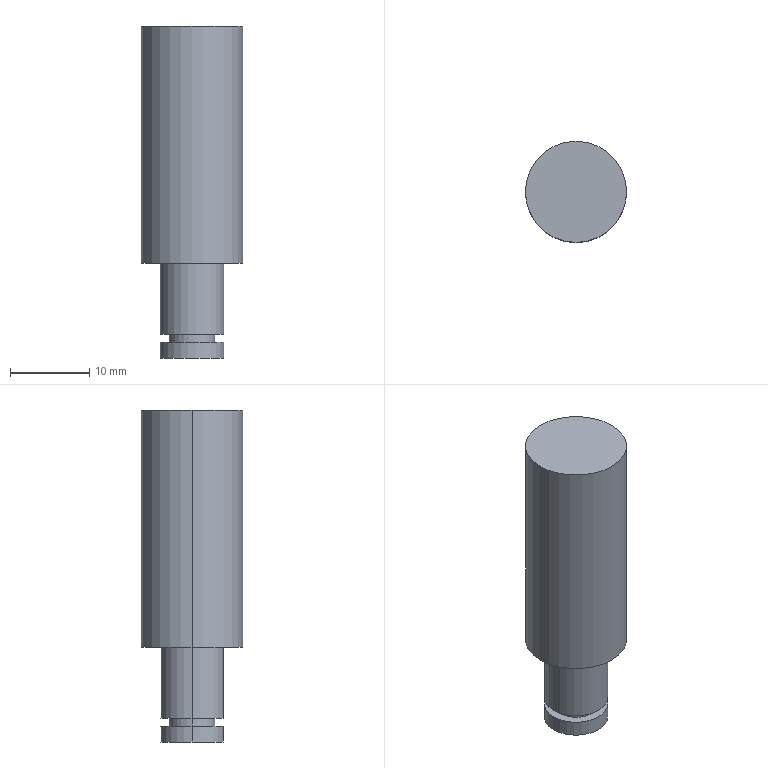Part | SolidWorks | features Revolution 1 | 1 solid | 13 faces | box 12.8 x 12.8 x 42 mm | volume 4440 mm3 | cylinder 8 | plane 5 | commonest cylinder face diameters 8 x4 5.8 x2 12.8 x2
STEP:
#1=CARTESIAN_POINT('',(-6.4,0.,42.));
#2=VERTEX_POINT('',#1);
#3=CARTESIAN_POINT('',(6.4,0.,42.));
#4=VERTEX_POINT('',#3);
#5=CARTESIAN_POINT('',(0.,0.,42.));
#6=DIRECTION('',(0.,0.,-1.));
#7=DIRECTION('',(-1.,0.,0.));
#8=AXIS2_PLACEMENT_3D('',#5,#6,#7);
#9=CIRCLE('',#8,6.4);
#10=EDGE_CURVE('',#2,#4,#9,.T.);
#11=ORIENTED_EDGE('',*,*,#10,.T.);
#12=CARTESIAN_POINT('',(6.4,0.,12.));
#13=VERTEX_POINT('',#12);
#14=CARTESIAN_POINT('',(6.4,0.,0.));
#15=DIRECTION('',(0.,0.,-1.));
#16=VECTOR('',#15,1000.);
#17=LINE('',#14,#16);
#18=EDGE_CURVE('',#4,#13,#17,.T.);
#19=ORIENTED_EDGE('',*,*,#18,.T.);
#20=CARTESIAN_POINT('',(-6.4,0.,12.));
#21=VERTEX_POINT('',#20);
#22=CARTESIAN_POINT('',(0.,0.,12.));
#23=DIRECTION('',(0.,0.,-1.));
#24=DIRECTION('',(-1.,0.,0.));
#25=AXIS2_PLACEMENT_3D('',#22,#23,#24);
#26=CIRCLE('',#25,6.4);
#27=EDGE_CURVE('',#21,#13,#26,.T.);
#28=ORIENTED_EDGE('',*,*,#27,.F.);
#29=CARTESIAN_POINT('',(-6.4,0.,0.));
#30=DIRECTION('',(0.,0.,-1.));
#31=VECTOR('',#30,1000.);
#32=LINE('',#29,#31);
#33=EDGE_CURVE('',#2,#21,#32,.T.);
#34=ORIENTED_EDGE('',*,*,#33,.F.);
#35=EDGE_LOOP('',(#11,#19,#28,#34));
#36=FACE_OUTER_BOUND('',#35,.T.);
#37=CARTESIAN_POINT('',(0.,0.,0.));
#38=DIRECTION('',(0.,0.,-1.));
#39=DIRECTION('',(-1.,0.,0.));
#40=AXIS2_PLACEMENT_3D('',#37,#38,#39);
#41=CYLINDRICAL_SURFACE('',#40,6.4);
#42=ADVANCED_FACE('',(#36),#41,.T.);
#43=CARTESIAN_POINT('',(-4.,0.,12.));
#44=VERTEX_POINT('',#43);
#45=CARTESIAN_POINT('',(4.,0.,12.));
#46=VERTEX_POINT('',#45);
#47=CARTESIAN_POINT('',(0.,0.,12.));
#48=DIRECTION('',(0.,0.,-1.));
#49=DIRECTION('',(-1.,0.,0.));
#50=AXIS2_PLACEMENT_3D('',#47,#48,#49);
#51=CIRCLE('',#50,4.);
#52=EDGE_CURVE('',#44,#46,#51,.T.);
#53=ORIENTED_EDGE('',*,*,#52,.T.);
#54=CARTESIAN_POINT('',(4.,0.,3.));
#55=VERTEX_POINT('',#54);
#56=CARTESIAN_POINT('',(4.,0.,0.));
#57=DIRECTION('',(0.,0.,-1.));
#58=VECTOR('',#57,1000.);
#59=LINE('',#56,#58);
#60=EDGE_CURVE('',#46,#55,#59,.T.);
#61=ORIENTED_EDGE('',*,*,#60,.T.);
#62=CARTESIAN_POINT('',(-4.,0.,3.));
#63=VERTEX_POINT('',#62);
#64=CARTESIAN_POINT('',(0.,0.,3.));
#65=DIRECTION('',(0.,0.,-1.));
#66=DIRECTION('',(-1.,0.,0.));
#67=AXIS2_PLACEMENT_3D('',#64,#65,#66);
#68=CIRCLE('',#67,4.);
#69=EDGE_CURVE('',#63,#55,#68,.T.);
#70=ORIENTED_EDGE('',*,*,#69,.F.);
#71=CARTESIAN_POINT('',(-4.,0.,0.));
#72=DIRECTION('',(0.,0.,-1.));
#73=VECTOR('',#72,1000.);
#74=LINE('',#71,#73);
#75=EDGE_CURVE('',#44,#63,#74,.T.);
#76=ORIENTED_EDGE('',*,*,#75,.F.);
#77=EDGE_LOOP('',(#53,#61,#70,#76));
#78=FACE_OUTER_BOUND('',#77,.T.);
#79=CARTESIAN_POINT('',(0.,0.,0.));
#80=DIRECTION('',(0.,0.,-1.));
#81=DIRECTION('',(-1.,0.,0.));
#82=AXIS2_PLACEMENT_3D('',#79,#80,#81);
#83=CYLINDRICAL_SURFACE('',#82,4.);
#84=ADVANCED_FACE('',(#78),#83,.T.);
#85=CARTESIAN_POINT('',(-2.9,0.,3.));
#86=VERTEX_POINT('',#85);
#87=CARTESIAN_POINT('',(2.9,0.,3.));
#88=VERTEX_POINT('',#87);
#89=CARTESIAN_POINT('',(0.,0.,3.));
#90=DIRECTION('',(0.,0.,-1.));
#91=DIRECTION('',(-1.,0.,0.));
#92=AXIS2_PLACEMENT_3D('',#89,#90,#91);
#93=CIRCLE('',#92,2.9);
#94=EDGE_CURVE('',#86,#88,#93,.T.);
#95=ORIENTED_EDGE('',*,*,#94,.T.);
#96=CARTESIAN_POINT('',(2.9,0.,2.));
#97=VERTEX_POINT('',#96);
#98=CARTESIAN_POINT('',(2.9,0.,0.));
#99=DIRECTION('',(0.,0.,-1.));
#100=VECTOR('',#99,1000.);
#101=LINE('',#98,#100);
#102=EDGE_CURVE('',#88,#97,#101,.T.);
#103=ORIENTED_EDGE('',*,*,#102,.T.);
#104=CARTESIAN_POINT('',(-2.9,0.,2.));
#105=VERTEX_POINT('',#104);
#106=CARTESIAN_POINT('',(0.,0.,2.));
#107=DIRECTION('',(0.,0.,-1.));
#108=DIRECTION('',(-1.,0.,0.));
#109=AXIS2_PLACEMENT_3D('',#106,#107,#108);
#110=CIRCLE('',#109,2.9);
#111=EDGE_CURVE('',#105,#97,#110,.T.);
#112=ORIENTED_EDGE('',*,*,#111,.F.);
#113=CARTESIAN_POINT('',(-2.9,0.,0.));
#114=DIRECTION('',(0.,0.,-1.));
#115=VECTOR('',#114,1000.);
#116=LINE('',#113,#115);
#117=EDGE_CURVE('',#86,#105,#116,.T.);
#118=ORIENTED_EDGE('',*,*,#117,.F.);
#119=EDGE_LOOP('',(#95,#103,#112,#118));
#120=FACE_OUTER_BOUND('',#119,.T.);
#121=CARTESIAN_POINT('',(0.,0.,0.));
#122=DIRECTION('',(0.,0.,-1.));
#123=DIRECTION('',(-1.,0.,0.));
#124=AXIS2_PLACEMENT_3D('',#121,#122,#123);
#125=CYLINDRICAL_SURFACE('',#124,2.9);
#126=ADVANCED_FACE('',(#120),#125,.T.);
#127=CARTESIAN_POINT('',(-4.,0.,2.));
#128=VERTEX_POINT('',#127);
#129=CARTESIAN_POINT('',(4.,0.,2.));
#130=VERTEX_POINT('',#129);
#131=CARTESIAN_POINT('',(0.,0.,2.));
#132=DIRECTION('',(0.,0.,-1.));
#133=DIRECTION('',(-1.,0.,0.));
#134=AXIS2_PLACEMENT_3D('',#131,#132,#133);
#135=CIRCLE('',#134,4.);
#136=EDGE_CURVE('',#128,#130,#135,.T.);
#137=ORIENTED_EDGE('',*,*,#136,.T.);
#138=CARTESIAN_POINT('',(4.,0.,0.));
#139=VERTEX_POINT('',#138);
#140=CARTESIAN_POINT('',(4.,0.,0.));
#141=DIRECTION('',(0.,0.,-1.));
#142=VECTOR('',#141,1000.);
#143=LINE('',#140,#142);
#144=EDGE_CURVE('',#130,#139,#143,.T.);
#145=ORIENTED_EDGE('',*,*,#144,.T.);
#146=CARTESIAN_POINT('',(-4.,0.,0.));
#147=VERTEX_POINT('',#146);
#148=CARTESIAN_POINT('',(0.,0.,0.));
#149=DIRECTION('',(0.,0.,-1.));
#150=DIRECTION('',(-1.,0.,0.));
#151=AXIS2_PLACEMENT_3D('',#148,#149,#150);
#152=CIRCLE('',#151,4.);
#153=EDGE_CURVE('',#147,#139,#152,.T.);
#154=ORIENTED_EDGE('',*,*,#153,.F.);
#155=CARTESIAN_POINT('',(-4.,0.,0.));
#156=DIRECTION('',(0.,0.,-1.));
#157=VECTOR('',#156,1000.);
#158=LINE('',#155,#157);
#159=EDGE_CURVE('',#128,#147,#158,.T.);
#160=ORIENTED_EDGE('',*,*,#159,.F.);
#161=EDGE_LOOP('',(#137,#145,#154,#160));
#162=FACE_OUTER_BOUND('',#161,.T.);
#163=CARTESIAN_POINT('',(0.,0.,0.));
#164=DIRECTION('',(0.,0.,-1.));
#165=DIRECTION('',(-1.,0.,0.));
#166=AXIS2_PLACEMENT_3D('',#163,#164,#165);
#167=CYLINDRICAL_SURFACE('',#166,4.);
#168=ADVANCED_FACE('',(#162),#167,.T.);
#169=ORIENTED_EDGE('',*,*,#153,.T.);
#170=CARTESIAN_POINT('',(0.,0.,0.));
#171=DIRECTION('',(0.,0.,-1.));
#172=DIRECTION('',(-1.,0.,0.));
#173=AXIS2_PLACEMENT_3D('',#170,#171,#172);
#174=CIRCLE('',#173,4.);
#175=EDGE_CURVE('',#139,#147,#174,.T.);
#176=ORIENTED_EDGE('',*,*,#175,.T.);
#177=EDGE_LOOP('',(#169,#176));
#178=FACE_OUTER_BOUND('',#177,.T.);
#179=CARTESIAN_POINT('',(0.,0.,0.));
#180=DIRECTION('',(0.,0.,-1.));
#181=DIRECTION('',(-1.,0.,0.));
#182=AXIS2_PLACEMENT_3D('',#179,#180,#181);
#183=PLANE('',#182);
#184=ADVANCED_FACE('',(#178),#183,.T.);
#185=ORIENTED_EDGE('',*,*,#144,.F.);
#186=CARTESIAN_POINT('',(0.,0.,2.));
#187=DIRECTION('',(0.,0.,-1.));
#188=DIRECTION('',(-1.,0.,0.));
#189=AXIS2_PLACEMENT_3D('',#186,#187,#188);
#190=CIRCLE('',#189,4.);
#191=EDGE_CURVE('',#130,#128,#190,.T.);
#192=ORIENTED_EDGE('',*,*,#191,.T.);
#193=ORIENTED_EDGE('',*,*,#159,.T.);
#194=ORIENTED_EDGE('',*,*,#175,.F.);
#195=EDGE_LOOP('',(#185,#192,#193,#194));
#196=FACE_OUTER_BOUND('',#195,.T.);
#197=CARTESIAN_POINT('',(0.,0.,0.));
#198=DIRECTION('',(0.,0.,-1.));
#199=DIRECTION('',(-1.,0.,0.));
#200=AXIS2_PLACEMENT_3D('',#197,#198,#199);
#201=CYLINDRICAL_SURFACE('',#200,4.);
#202=ADVANCED_FACE('',(#196),#201,.T.);
#203=ORIENTED_EDGE('',*,*,#111,.T.);
#204=CARTESIAN_POINT('',(0.,0.,2.));
#205=DIRECTION('',(0.,0.,-1.));
#206=DIRECTION('',(-1.,0.,0.));
#207=AXIS2_PLACEMENT_3D('',#204,#205,#206);
#208=CIRCLE('',#207,2.9);
#209=EDGE_CURVE('',#97,#105,#208,.T.);
#210=ORIENTED_EDGE('',*,*,#209,.T.);
#211=EDGE_LOOP('',(#203,#210));
#212=FACE_BOUND('',#211,.T.);
#213=ORIENTED_EDGE('',*,*,#136,.F.);
#214=ORIENTED_EDGE('',*,*,#191,.F.);
#215=EDGE_LOOP('',(#213,#214));
#216=FACE_OUTER_BOUND('',#215,.T.);
#217=CARTESIAN_POINT('',(-4.,0.,2.));
#218=DIRECTION('',(0.,0.,1.));
#219=DIRECTION('',(1.,0.,0.));
#220=AXIS2_PLACEMENT_3D('',#217,#218,#219);
#221=PLANE('',#220);
#222=ADVANCED_FACE('',(#212,#216),#221,.T.);
#223=ORIENTED_EDGE('',*,*,#102,.F.);
#224=CARTESIAN_POINT('',(0.,0.,3.));
#225=DIRECTION('',(0.,0.,-1.));
#226=DIRECTION('',(-1.,0.,0.));
#227=AXIS2_PLACEMENT_3D('',#224,#225,#226);
#228=CIRCLE('',#227,2.9);
#229=EDGE_CURVE('',#88,#86,#228,.T.);
#230=ORIENTED_EDGE('',*,*,#229,.T.);
#231=ORIENTED_EDGE('',*,*,#117,.T.);
#232=ORIENTED_EDGE('',*,*,#209,.F.);
#233=EDGE_LOOP('',(#223,#230,#231,#232));
#234=FACE_OUTER_BOUND('',#233,.T.);
#235=CARTESIAN_POINT('',(0.,0.,0.));
#236=DIRECTION('',(0.,0.,-1.));
#237=DIRECTION('',(-1.,0.,0.));
#238=AXIS2_PLACEMENT_3D('',#235,#236,#237);
#239=CYLINDRICAL_SURFACE('',#238,2.9);
#240=ADVANCED_FACE('',(#234),#239,.T.);
#241=ORIENTED_EDGE('',*,*,#69,.T.);
#242=CARTESIAN_POINT('',(0.,0.,3.));
#243=DIRECTION('',(0.,0.,-1.));
#244=DIRECTION('',(-1.,0.,0.));
#245=AXIS2_PLACEMENT_3D('',#242,#243,#244);
#246=CIRCLE('',#245,4.);
#247=EDGE_CURVE('',#55,#63,#246,.T.);
#248=ORIENTED_EDGE('',*,*,#247,.T.);
#249=EDGE_LOOP('',(#241,#248));
#250=FACE_OUTER_BOUND('',#249,.T.);
#251=ORIENTED_EDGE('',*,*,#94,.F.);
#252=ORIENTED_EDGE('',*,*,#229,.F.);
#253=EDGE_LOOP('',(#251,#252));
#254=FACE_BOUND('',#253,.T.);
#255=CARTESIAN_POINT('',(-2.9,0.,3.));
#256=DIRECTION('',(0.,0.,-1.));
#257=DIRECTION('',(-1.,0.,0.));
#258=AXIS2_PLACEMENT_3D('',#255,#256,#257);
#259=PLANE('',#258);
#260=ADVANCED_FACE('',(#250,#254),#259,.T.);
#261=ORIENTED_EDGE('',*,*,#60,.F.);
#262=CARTESIAN_POINT('',(0.,0.,12.));
#263=DIRECTION('',(0.,0.,-1.));
#264=DIRECTION('',(-1.,0.,0.));
#265=AXIS2_PLACEMENT_3D('',#262,#263,#264);
#266=CIRCLE('',#265,4.);
#267=EDGE_CURVE('',#46,#44,#266,.T.);
#268=ORIENTED_EDGE('',*,*,#267,.T.);
#269=ORIENTED_EDGE('',*,*,#75,.T.);
#270=ORIENTED_EDGE('',*,*,#247,.F.);
#271=EDGE_LOOP('',(#261,#268,#269,#270));
#272=FACE_OUTER_BOUND('',#271,.T.);
#273=CARTESIAN_POINT('',(0.,0.,0.));
#274=DIRECTION('',(0.,0.,-1.));
#275=DIRECTION('',(-1.,0.,0.));
#276=AXIS2_PLACEMENT_3D('',#273,#274,#275);
#277=CYLINDRICAL_SURFACE('',#276,4.);
#278=ADVANCED_FACE('',(#272),#277,.T.);
#279=ORIENTED_EDGE('',*,*,#27,.T.);
#280=CARTESIAN_POINT('',(0.,0.,12.));
#281=DIRECTION('',(0.,0.,-1.));
#282=DIRECTION('',(-1.,0.,0.));
#283=AXIS2_PLACEMENT_3D('',#280,#281,#282);
#284=CIRCLE('',#283,6.4);
#285=EDGE_CURVE('',#13,#21,#284,.T.);
#286=ORIENTED_EDGE('',*,*,#285,.T.);
#287=EDGE_LOOP('',(#279,#286));
#288=FACE_OUTER_BOUND('',#287,.T.);
#289=ORIENTED_EDGE('',*,*,#52,.F.);
#290=ORIENTED_EDGE('',*,*,#267,.F.);
#291=EDGE_LOOP('',(#289,#290));
#292=FACE_BOUND('',#291,.T.);
#293=CARTESIAN_POINT('',(-4.,0.,12.));
#294=DIRECTION('',(0.,0.,-1.));
#295=DIRECTION('',(-1.,0.,0.));
#296=AXIS2_PLACEMENT_3D('',#293,#294,#295);
#297=PLANE('',#296);
#298=ADVANCED_FACE('',(#288,#292),#297,.T.);
#299=ORIENTED_EDGE('',*,*,#18,.F.);
#300=CARTESIAN_POINT('',(0.,0.,42.));
#301=DIRECTION('',(0.,0.,-1.));
#302=DIRECTION('',(-1.,0.,0.));
#303=AXIS2_PLACEMENT_3D('',#300,#301,#302);
#304=CIRCLE('',#303,6.4);
#305=EDGE_CURVE('',#4,#2,#304,.T.);
#306=ORIENTED_EDGE('',*,*,#305,.T.);
#307=ORIENTED_EDGE('',*,*,#33,.T.);
#308=ORIENTED_EDGE('',*,*,#285,.F.);
#309=EDGE_LOOP('',(#299,#306,#307,#308));
#310=FACE_OUTER_BOUND('',#309,.T.);
#311=CARTESIAN_POINT('',(0.,0.,0.));
#312=DIRECTION('',(0.,0.,-1.));
#313=DIRECTION('',(-1.,0.,0.));
#314=AXIS2_PLACEMENT_3D('',#311,#312,#313);
#315=CYLINDRICAL_SURFACE('',#314,6.4);
#316=ADVANCED_FACE('',(#310),#315,.T.);
#317=ORIENTED_EDGE('',*,*,#10,.F.);
#318=ORIENTED_EDGE('',*,*,#305,.F.);
#319=EDGE_LOOP('',(#317,#318));
#320=FACE_OUTER_BOUND('',#319,.T.);
#321=CARTESIAN_POINT('',(-6.4,0.,42.));
#322=DIRECTION('',(0.,0.,1.));
#323=DIRECTION('',(1.,0.,0.));
#324=AXIS2_PLACEMENT_3D('',#321,#322,#323);
#325=PLANE('',#324);
#326=ADVANCED_FACE('',(#320),#325,.T.);
#327=CLOSED_SHELL('',(#42,#84,#126,#168,#184,#202,#222,#240,#260,#278,#298,#316,#326));
#328=MANIFOLD_SOLID_BREP('',#327);
#329=CARTESIAN_POINT('',(0.,0.,0.));
#330=DIRECTION('',(0.,0.,1.));
#331=DIRECTION('',(1.,0.,0.));
#332=AXIS2_PLACEMENT_3D('',#329,#330,#331);
#333=(LENGTH_UNIT()NAMED_UNIT(*)SI_UNIT(.MILLI.,.METRE.));
#334=UNCERTAINTY_MEASURE_WITH_UNIT(LENGTH_MEASURE(0.00001),#333,'','');
#335=(NAMED_UNIT(*)PLANE_ANGLE_UNIT()SI_UNIT($,.RADIAN.));
#336=(NAMED_UNIT(*)SI_UNIT($,.STERADIAN.)SOLID_ANGLE_UNIT());
#337=(GEOMETRIC_REPRESENTATION_CONTEXT(3)GLOBAL_UNCERTAINTY_ASSIGNED_CONTEXT((#334))GLOBAL_UNIT_ASSIGNED_CONTEXT((#333,#335,#336))REPRESENTATION_CONTEXT('',''));
#338=ADVANCED_BREP_SHAPE_REPRESENTATION('',(#328,#332),#337);